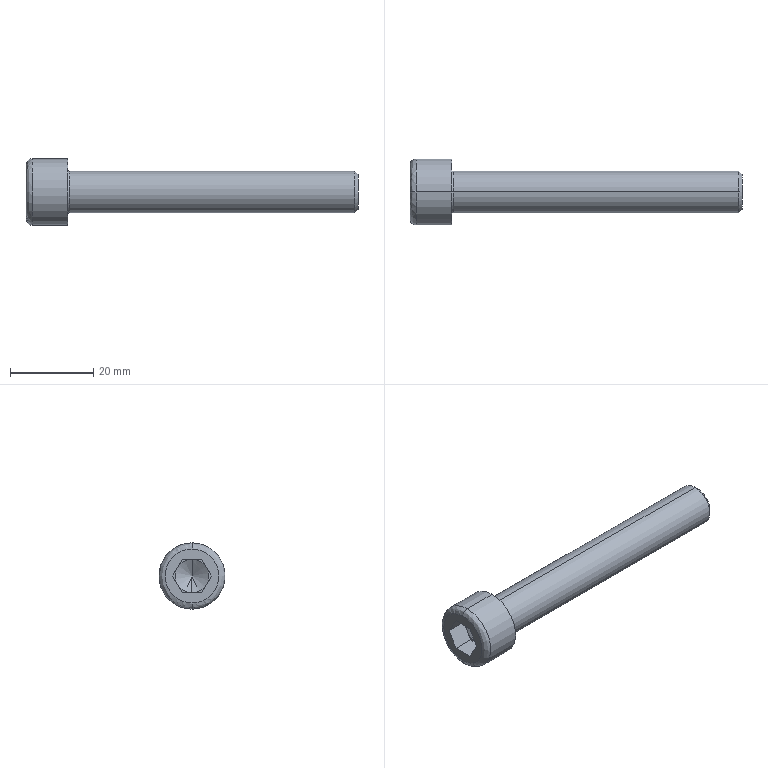Part | SolidWorks | features BaseBody 1 | 1 solid | 27 faces | box 80 x 16 x 16 mm | volume 7150 mm3 | plane 15 | spline 4 | cylinder 4 | cone 4 | commonest cylinder face diameters 10 x2 16 x2
STEP:
#1=CARTESIAN_POINT('',(10.,0.,5.4));
#2=VERTEX_POINT('',#1);
#3=CARTESIAN_POINT('',(10.,0.,-5.4));
#4=VERTEX_POINT('',#3);
#5=CARTESIAN_POINT('',(10.,0.,5.4));
#6=CARTESIAN_POINT('',(10.,0.1651,5.4));
#7=CARTESIAN_POINT('',(10.,0.4117,5.389));
#8=CARTESIAN_POINT('',(10.,0.6977,5.356));
#9=CARTESIAN_POINT('',(10.,0.8403,5.334));
#10=CARTESIAN_POINT('',(10.,0.9013,5.324));
#11=CARTESIAN_POINT('',(10.,0.942,5.317));
#12=CARTESIAN_POINT('',(10.,0.9611,5.314));
#13=CARTESIAN_POINT('',(10.,1.155,5.278));
#14=CARTESIAN_POINT('',(10.,1.409,5.218));
#15=CARTESIAN_POINT('',(10.,1.7,5.127));
#16=CARTESIAN_POINT('',(10.,1.824,5.083));
#17=CARTESIAN_POINT('',(10.,1.906,5.053));
#18=CARTESIAN_POINT('',(10.,1.945,5.038));
#19=CARTESIAN_POINT('',(10.,2.157,4.954));
#20=CARTESIAN_POINT('',(10.,2.405,4.841));
#21=CARTESIAN_POINT('',(10.,2.644,4.709));
#22=CARTESIAN_POINT('',(10.,2.801,4.618));
#23=CARTESIAN_POINT('',(10.,2.877,4.571));
#24=CARTESIAN_POINT('',(10.,3.267,4.316));
#25=CARTESIAN_POINT('',(10.,3.555,4.082));
#26=CARTESIAN_POINT('',(10.,3.95,3.687));
#27=CARTESIAN_POINT('',(10.,4.137,3.48));
#28=CARTESIAN_POINT('',(10.,4.306,3.26));
#29=CARTESIAN_POINT('',(10.,4.416,3.11));
#30=CARTESIAN_POINT('',(10.,4.47,3.031));
#31=CARTESIAN_POINT('',(10.,4.62,2.802));
#32=CARTESIAN_POINT('',(10.,4.757,2.567));
#33=CARTESIAN_POINT('',(10.,4.896,2.281));
#34=CARTESIAN_POINT('',(10.,4.951,2.156));
#35=CARTESIAN_POINT('',(10.,4.987,2.072));
#36=CARTESIAN_POINT('',(10.,5.005,2.028));
#37=CARTESIAN_POINT('',(10.,5.085,1.825));
#38=CARTESIAN_POINT('',(10.,5.17,1.577));
#39=CARTESIAN_POINT('',(10.,5.247,1.282));
#40=CARTESIAN_POINT('',(10.,5.28,1.133));
#41=CARTESIAN_POINT('',(10.,5.293,1.069));
#42=CARTESIAN_POINT('',(10.,5.302,1.026));
#43=CARTESIAN_POINT('',(10.,5.306,1.003));
#44=CARTESIAN_POINT('',(10.,5.37,0.6582));
#45=CARTESIAN_POINT('',(10.,5.4,0.3299));
#46=CARTESIAN_POINT('',(10.,5.4,-0.165));
#47=CARTESIAN_POINT('',(10.,5.389,-0.4115));
#48=CARTESIAN_POINT('',(10.,5.356,-0.6976));
#49=CARTESIAN_POINT('',(10.,5.335,-0.8402));
#50=CARTESIAN_POINT('',(10.,5.324,-0.9013));
#51=CARTESIAN_POINT('',(10.,5.317,-0.9419));
#52=CARTESIAN_POINT('',(10.,5.314,-0.9611));
#53=CARTESIAN_POINT('',(10.,5.278,-1.155));
#54=CARTESIAN_POINT('',(10.,5.218,-1.409));
#55=CARTESIAN_POINT('',(10.,5.127,-1.7));
#56=CARTESIAN_POINT('',(10.,5.083,-1.824));
#57=CARTESIAN_POINT('',(10.,5.053,-1.906));
#58=CARTESIAN_POINT('',(10.,5.038,-1.945));
#59=CARTESIAN_POINT('',(10.,4.954,-2.157));
#60=CARTESIAN_POINT('',(10.,4.841,-2.405));
#61=CARTESIAN_POINT('',(10.,4.709,-2.644));
#62=CARTESIAN_POINT('',(10.,4.618,-2.801));
#63=CARTESIAN_POINT('',(10.,4.571,-2.877));
#64=CARTESIAN_POINT('',(10.,4.316,-3.267));
#65=CARTESIAN_POINT('',(10.,4.082,-3.555));
#66=CARTESIAN_POINT('',(10.,3.687,-3.95));
#67=CARTESIAN_POINT('',(10.,3.48,-4.137));
#68=CARTESIAN_POINT('',(10.,3.26,-4.306));
#69=CARTESIAN_POINT('',(10.,3.11,-4.416));
#70=CARTESIAN_POINT('',(10.,3.031,-4.47));
#71=CARTESIAN_POINT('',(10.,2.802,-4.62));
#72=CARTESIAN_POINT('',(10.,2.567,-4.757));
#73=CARTESIAN_POINT('',(10.,2.281,-4.896));
#74=CARTESIAN_POINT('',(10.,2.156,-4.951));
#75=CARTESIAN_POINT('',(10.,2.072,-4.987));
#76=CARTESIAN_POINT('',(10.,2.028,-5.005));
#77=CARTESIAN_POINT('',(10.,1.825,-5.085));
#78=CARTESIAN_POINT('',(10.,1.577,-5.17));
#79=CARTESIAN_POINT('',(10.,1.282,-5.247));
#80=CARTESIAN_POINT('',(10.,1.133,-5.28));
#81=CARTESIAN_POINT('',(10.,1.069,-5.293));
#82=CARTESIAN_POINT('',(10.,1.026,-5.302));
#83=CARTESIAN_POINT('',(10.,1.003,-5.306));
#84=CARTESIAN_POINT('',(10.,0.658,-5.37));
#85=CARTESIAN_POINT('',(10.,0.3305,-5.4));
#86=CARTESIAN_POINT('',(10.,0.,-5.4));
#87=B_SPLINE_CURVE_WITH_KNOTS('',3,(#5,#6,#7,#8,#9,#10,#11,#12,#13,#14,#15,#16,#17,#18,#19,#20,#21,#22,#23,#24,#25,#26,#27,#28,#29,#30,#31,#32,#33,#34,#35,#36,#37,#38,#39,#40,#41,#42,#43,#44,#45,#46,#47,#48,#49,#50,#51,#52,#53,#54,#55,#56,#57,#58,#59,#60,#61,#62,#63,#64,#65,#66,#67,#68,#69,#70,#71,#72,#73,#74,#75,#76,#77,#78,#79,#80,#81,#82,#83,#84,#85,#86),.UNSPECIFIED.,.F.,.F.,(4,1,1,1,2,2,1,1,2,2,1,2,2,2,1,2,2,1,1,2,2,1,1,1,2,2,2,1,1,1,2,2,1,1,2,2,1,2,2,2,1,2,2,1,1,2,2,1,1,1,2,2,4),(0.,0.03125,0.04687,0.05469,0.05859,0.0625,0.09375,0.1094,0.1172,0.125,0.1562,0.1719,0.1875,0.25,0.2812,0.2969,0.3125,0.3437,0.3594,0.3672,0.375,0.4062,0.4219,0.4297,0.4336,0.4375,0.5,0.5312,0.5469,0.5547,0.5586,0.5625,0.5937,0.6094,0.6172,0.625,0.6562,0.6719,0.6875,0.75,0.7813,0.7969,0.8125,0.8438,0.8594,0.8672,0.875,0.9063,0.9219,0.9297,0.9336,0.9375,1.),.UNSPECIFIED.);
#88=EDGE_CURVE('',#2,#4,#87,.T.);
#89=ORIENTED_EDGE('',*,*,#88,.F.);
#90=CARTESIAN_POINT('',(10.4,0.,5.));
#91=VERTEX_POINT('',#90);
#92=CARTESIAN_POINT('',(10.4,0.,5.4));
#93=DIRECTION('',(0.,-1.,0.));
#94=DIRECTION('',(0.,0.,1.));
#95=AXIS2_PLACEMENT_3D('',#92,#93,#94);
#96=CIRCLE('',#95,0.4);
#97=EDGE_CURVE('',#2,#91,#96,.T.);
#98=ORIENTED_EDGE('',*,*,#97,.T.);
#99=CARTESIAN_POINT('',(10.4,0.,-5.));
#100=VERTEX_POINT('',#99);
#101=CARTESIAN_POINT('',(10.4,0.,0.));
#102=DIRECTION('',(1.,0.,0.));
#103=DIRECTION('',(0.,0.,1.));
#104=AXIS2_PLACEMENT_3D('',#101,#102,#103);
#105=CIRCLE('',#104,5.);
#106=EDGE_CURVE('',#100,#91,#105,.T.);
#107=ORIENTED_EDGE('',*,*,#106,.F.);
#108=CARTESIAN_POINT('',(10.4,0.,-5.4));
#109=DIRECTION('',(0.,1.,0.));
#110=DIRECTION('',(0.,0.,-1.));
#111=AXIS2_PLACEMENT_3D('',#108,#109,#110);
#112=CIRCLE('',#111,0.4);
#113=EDGE_CURVE('',#4,#100,#112,.T.);
#114=ORIENTED_EDGE('',*,*,#113,.F.);
#115=EDGE_LOOP('',(#89,#98,#107,#114));
#116=FACE_OUTER_BOUND('',#115,.T.);
#117=CARTESIAN_POINT('',(10.,0.,-5.4));
#118=CARTESIAN_POINT('',(10.,10.8,-5.4));
#119=CARTESIAN_POINT('',(10.,10.8,5.4));
#120=CARTESIAN_POINT('',(10.,0.,5.4));
#121=CARTESIAN_POINT('',(10.,0.,-5.166));
#122=CARTESIAN_POINT('',(10.,10.331,-5.166));
#123=CARTESIAN_POINT('',(10.,10.331,5.166));
#124=CARTESIAN_POINT('',(10.,0.,5.166));
#125=CARTESIAN_POINT('',(10.166,0.,-5.));
#126=CARTESIAN_POINT('',(10.166,10.,-5.));
#127=CARTESIAN_POINT('',(10.166,10.,5.));
#128=CARTESIAN_POINT('',(10.166,0.,5.));
#129=CARTESIAN_POINT('',(10.4,0.,-5.));
#130=CARTESIAN_POINT('',(10.4,10.,-5.));
#131=CARTESIAN_POINT('',(10.4,10.,5.));
#132=CARTESIAN_POINT('',(10.4,0.,5.));
#133=(BOUNDED_SURFACE()B_SPLINE_SURFACE(3,3,((#117,#118,#119,#120),(#121,#122,#123,#124),(#125,#126,#127,#128),(#129,#130,#131,#132)),.UNSPECIFIED.,.F.,.F.,.F.)B_SPLINE_SURFACE_WITH_KNOTS((4,4),(4,4),(0.,1.),(0.,1.),.UNSPECIFIED.)GEOMETRIC_REPRESENTATION_ITEM()RATIONAL_B_SPLINE_SURFACE(((1.,0.3333,0.3333,1.),(0.8047,0.2682,0.2682,0.8047),(0.8047,0.2682,0.2682,0.8047),(1.,0.3333,0.3333,1.)))REPRESENTATION_ITEM('')SURFACE());
#134=ADVANCED_FACE('',(#116),#133,.F.);
#135=CARTESIAN_POINT('',(0.,0.,6.5));
#136=VERTEX_POINT('',#135);
#137=CARTESIAN_POINT('',(0.,0.,-6.5));
#138=VERTEX_POINT('',#137);
#139=CARTESIAN_POINT('',(0.,0.,6.5));
#140=CARTESIAN_POINT('',(0.,-13.,6.5));
#141=CARTESIAN_POINT('',(0.,-13.,-6.5));
#142=CARTESIAN_POINT('',(0.,0.,-6.5));
#143=(BOUNDED_CURVE()B_SPLINE_CURVE(3,(#139,#140,#141,#142),.UNSPECIFIED.,.F.,.F.)B_SPLINE_CURVE_WITH_KNOTS((4,4),(0.,1.),.UNSPECIFIED.)CURVE()GEOMETRIC_REPRESENTATION_ITEM()RATIONAL_B_SPLINE_CURVE((1.,0.3333,0.3333,1.))REPRESENTATION_ITEM(''));
#144=EDGE_CURVE('',#136,#138,#143,.T.);
#145=ORIENTED_EDGE('',*,*,#144,.T.);
#146=CARTESIAN_POINT('',(1.5,0.,-8.));
#147=VERTEX_POINT('',#146);
#148=CARTESIAN_POINT('',(1.5,0.,-6.5));
#149=DIRECTION('',(0.,-1.,0.));
#150=DIRECTION('',(0.,0.,-1.));
#151=AXIS2_PLACEMENT_3D('',#148,#149,#150);
#152=CIRCLE('',#151,1.5);
#153=EDGE_CURVE('',#138,#147,#152,.T.);
#154=ORIENTED_EDGE('',*,*,#153,.T.);
#155=CARTESIAN_POINT('',(1.5,0.,8.));
#156=VERTEX_POINT('',#155);
#157=CARTESIAN_POINT('',(1.5,0.,0.));
#158=DIRECTION('',(1.,0.,0.));
#159=DIRECTION('',(0.,0.,1.));
#160=AXIS2_PLACEMENT_3D('',#157,#158,#159);
#161=CIRCLE('',#160,8.);
#162=EDGE_CURVE('',#156,#147,#161,.T.);
#163=ORIENTED_EDGE('',*,*,#162,.F.);
#164=CARTESIAN_POINT('',(1.5,0.,6.5));
#165=DIRECTION('',(0.,1.,0.));
#166=DIRECTION('',(0.,0.,1.));
#167=AXIS2_PLACEMENT_3D('',#164,#165,#166);
#168=CIRCLE('',#167,1.5);
#169=EDGE_CURVE('',#136,#156,#168,.T.);
#170=ORIENTED_EDGE('',*,*,#169,.F.);
#171=EDGE_LOOP('',(#145,#154,#163,#170));
#172=FACE_OUTER_BOUND('',#171,.T.);
#173=CARTESIAN_POINT('',(0.,0.,-6.5));
#174=CARTESIAN_POINT('',(0.,-13.,-6.5));
#175=CARTESIAN_POINT('',(0.,-13.,6.5));
#176=CARTESIAN_POINT('',(0.,0.,6.5));
#177=CARTESIAN_POINT('',(0.,0.,-7.379));
#178=CARTESIAN_POINT('',(0.,-14.757,-7.379));
#179=CARTESIAN_POINT('',(0.,-14.757,7.379));
#180=CARTESIAN_POINT('',(0.,0.,7.379));
#181=CARTESIAN_POINT('',(0.6213,0.,-8.));
#182=CARTESIAN_POINT('',(0.6213,-16.,-8.));
#183=CARTESIAN_POINT('',(0.6213,-16.,8.));
#184=CARTESIAN_POINT('',(0.6213,0.,8.));
#185=CARTESIAN_POINT('',(1.5,0.,-8.));
#186=CARTESIAN_POINT('',(1.5,-16.,-8.));
#187=CARTESIAN_POINT('',(1.5,-16.,8.));
#188=CARTESIAN_POINT('',(1.5,0.,8.));
#189=(BOUNDED_SURFACE()B_SPLINE_SURFACE(3,3,((#173,#174,#175,#176),(#177,#178,#179,#180),(#181,#182,#183,#184),(#185,#186,#187,#188)),.UNSPECIFIED.,.F.,.F.,.F.)B_SPLINE_SURFACE_WITH_KNOTS((4,4),(4,4),(0.,1.),(0.,1.),.UNSPECIFIED.)GEOMETRIC_REPRESENTATION_ITEM()RATIONAL_B_SPLINE_SURFACE(((1.,0.3333,0.3333,1.),(0.8047,0.2682,0.2682,0.8047),(0.8047,0.2682,0.2682,0.8047),(1.,0.3333,0.3333,1.)))REPRESENTATION_ITEM('')SURFACE());
#190=ADVANCED_FACE('',(#172),#189,.T.);
#191=CARTESIAN_POINT('',(79.172,0.,5.));
#192=VERTEX_POINT('',#191);
#193=CARTESIAN_POINT('',(79.172,0.,-5.));
#194=VERTEX_POINT('',#193);
#195=CARTESIAN_POINT('',(79.172,0.,0.));
#196=DIRECTION('',(-1.,0.,0.));
#197=DIRECTION('',(0.,0.,1.));
#198=AXIS2_PLACEMENT_3D('',#195,#196,#197);
#199=CIRCLE('',#198,5.);
#200=EDGE_CURVE('',#192,#194,#199,.T.);
#201=ORIENTED_EDGE('',*,*,#200,.T.);
#202=CARTESIAN_POINT('',(-31.75,0.,-5.));
#203=DIRECTION('',(-1.,0.,0.));
#204=VECTOR('',#203,1000.);
#205=LINE('',#202,#204);
#206=EDGE_CURVE('',#194,#100,#205,.T.);
#207=ORIENTED_EDGE('',*,*,#206,.T.);
#208=ORIENTED_EDGE('',*,*,#106,.T.);
#209=CARTESIAN_POINT('',(-31.75,0.,5.));
#210=DIRECTION('',(-1.,0.,0.));
#211=VECTOR('',#210,1000.);
#212=LINE('',#209,#211);
#213=EDGE_CURVE('',#192,#91,#212,.T.);
#214=ORIENTED_EDGE('',*,*,#213,.F.);
#215=EDGE_LOOP('',(#201,#207,#208,#214));
#216=FACE_OUTER_BOUND('',#215,.T.);
#217=CARTESIAN_POINT('',(-31.75,0.,0.));
#218=DIRECTION('',(-1.,0.,0.));
#219=DIRECTION('',(0.,0.,1.));
#220=AXIS2_PLACEMENT_3D('',#217,#218,#219);
#221=CYLINDRICAL_SURFACE('',#220,5.);
#222=ADVANCED_FACE('',(#216),#221,.T.);
#223=CARTESIAN_POINT('',(80.,0.,4.172));
#224=VERTEX_POINT('',#223);
#225=CARTESIAN_POINT('',(80.,0.,-4.172));
#226=VERTEX_POINT('',#225);
#227=CARTESIAN_POINT('',(80.,0.,0.));
#228=DIRECTION('',(-1.,0.,0.));
#229=DIRECTION('',(0.,0.,1.));
#230=AXIS2_PLACEMENT_3D('',#227,#228,#229);
#231=CIRCLE('',#230,4.172);
#232=EDGE_CURVE('',#224,#226,#231,.T.);
#233=ORIENTED_EDGE('',*,*,#232,.T.);
#234=CARTESIAN_POINT('',(79.172,0.,-5.));
#235=DIRECTION('',(-0.7071,0.,-0.7071));
#236=VECTOR('',#235,1000.);
#237=LINE('',#234,#236);
#238=EDGE_CURVE('',#226,#194,#237,.T.);
#239=ORIENTED_EDGE('',*,*,#238,.T.);
#240=ORIENTED_EDGE('',*,*,#200,.F.);
#241=CARTESIAN_POINT('',(79.172,0.,5.));
#242=DIRECTION('',(-0.7071,0.,0.7071));
#243=VECTOR('',#242,1000.);
#244=LINE('',#241,#243);
#245=EDGE_CURVE('',#224,#192,#244,.T.);
#246=ORIENTED_EDGE('',*,*,#245,.F.);
#247=EDGE_LOOP('',(#233,#239,#240,#246));
#248=FACE_OUTER_BOUND('',#247,.T.);
#249=CARTESIAN_POINT('',(79.172,0.,0.));
#250=DIRECTION('',(-1.,0.,0.));
#251=DIRECTION('',(0.,0.,1.));
#252=AXIS2_PLACEMENT_3D('',#249,#250,#251);
#253=CONICAL_SURFACE('',#252,5.,0.7854);
#254=ADVANCED_FACE('',(#248),#253,.T.);
#255=CARTESIAN_POINT('',(10.,0.,-8.));
#256=VERTEX_POINT('',#255);
#257=CARTESIAN_POINT('',(10.,0.,8.));
#258=VERTEX_POINT('',#257);
#259=CARTESIAN_POINT('',(10.,0.,0.));
#260=DIRECTION('',(1.,0.,0.));
#261=DIRECTION('',(0.,0.,1.));
#262=AXIS2_PLACEMENT_3D('',#259,#260,#261);
#263=CIRCLE('',#262,8.);
#264=EDGE_CURVE('',#256,#258,#263,.T.);
#265=ORIENTED_EDGE('',*,*,#264,.F.);
#266=CARTESIAN_POINT('',(-31.75,0.,-8.));
#267=DIRECTION('',(-1.,0.,0.));
#268=VECTOR('',#267,1000.);
#269=LINE('',#266,#268);
#270=EDGE_CURVE('',#256,#147,#269,.T.);
#271=ORIENTED_EDGE('',*,*,#270,.T.);
#272=CARTESIAN_POINT('',(1.5,0.,0.));
#273=DIRECTION('',(1.,0.,0.));
#274=DIRECTION('',(0.,0.,1.));
#275=AXIS2_PLACEMENT_3D('',#272,#273,#274);
#276=CIRCLE('',#275,8.);
#277=EDGE_CURVE('',#147,#156,#276,.T.);
#278=ORIENTED_EDGE('',*,*,#277,.T.);
#279=CARTESIAN_POINT('',(-31.75,0.,8.));
#280=DIRECTION('',(-1.,0.,0.));
#281=VECTOR('',#280,1000.);
#282=LINE('',#279,#281);
#283=EDGE_CURVE('',#258,#156,#282,.T.);
#284=ORIENTED_EDGE('',*,*,#283,.F.);
#285=EDGE_LOOP('',(#265,#271,#278,#284));
#286=FACE_OUTER_BOUND('',#285,.T.);
#287=CARTESIAN_POINT('',(-31.75,0.,0.));
#288=DIRECTION('',(-1.,0.,0.));
#289=DIRECTION('',(0.,0.,1.));
#290=AXIS2_PLACEMENT_3D('',#287,#288,#289);
#291=CYLINDRICAL_SURFACE('',#290,8.);
#292=ADVANCED_FACE('',(#286),#291,.T.);
#293=CARTESIAN_POINT('',(7.343,0.,0.));
#294=VERTEX_POINT('',#293);
#295=CARTESIAN_POINT('',(5.,0.,4.057));
#296=VERTEX_POINT('',#295);
#297=CARTESIAN_POINT('',(5.,0.,4.057));
#298=DIRECTION('',(-0.5,0.,0.866));
#299=VECTOR('',#298,1000.);
#300=LINE('',#297,#299);
#301=EDGE_CURVE('',#294,#296,#300,.T.);
#302=ORIENTED_EDGE('',*,*,#301,.F.);
#303=CARTESIAN_POINT('',(5.,0.,-4.057));
#304=VERTEX_POINT('',#303);
#305=CARTESIAN_POINT('',(5.,0.,-4.057));
#306=DIRECTION('',(-0.5,0.,-0.866));
#307=VECTOR('',#306,1000.);
#308=LINE('',#305,#307);
#309=EDGE_CURVE('',#294,#304,#308,.T.);
#310=ORIENTED_EDGE('',*,*,#309,.T.);
#311=CARTESIAN_POINT('',(5.,-3.514,-2.029));
#312=VERTEX_POINT('',#311);
#313=CARTESIAN_POINT('',(5.,0.,0.));
#314=DIRECTION('',(-1.,0.,0.));
#315=DIRECTION('',(0.,0.,1.));
#316=AXIS2_PLACEMENT_3D('',#313,#314,#315);
#317=CIRCLE('',#316,4.057);
#318=EDGE_CURVE('',#304,#312,#317,.T.);
#319=ORIENTED_EDGE('',*,*,#318,.T.);
#320=CARTESIAN_POINT('',(5.,-3.514,2.029));
#321=VERTEX_POINT('',#320);
#322=CARTESIAN_POINT('',(5.,0.,0.));
#323=DIRECTION('',(-1.,0.,0.));
#324=DIRECTION('',(0.,0.,1.));
#325=AXIS2_PLACEMENT_3D('',#322,#323,#324);
#326=CIRCLE('',#325,4.057);
#327=EDGE_CURVE('',#312,#321,#326,.T.);
#328=ORIENTED_EDGE('',*,*,#327,.T.);
#329=CARTESIAN_POINT('',(5.,0.,0.));
#330=DIRECTION('',(-1.,0.,0.));
#331=DIRECTION('',(0.,0.,1.));
#332=AXIS2_PLACEMENT_3D('',#329,#330,#331);
#333=CIRCLE('',#332,4.057);
#334=EDGE_CURVE('',#321,#296,#333,.T.);
#335=ORIENTED_EDGE('',*,*,#334,.T.);
#336=EDGE_LOOP('',(#302,#310,#319,#328,#335));
#337=FACE_OUTER_BOUND('',#336,.T.);
#338=CARTESIAN_POINT('',(5.,0.,0.));
#339=DIRECTION('',(-1.,0.,0.));
#340=DIRECTION('',(0.,0.,1.));
#341=AXIS2_PLACEMENT_3D('',#338,#339,#340);
#342=CONICAL_SURFACE('',#341,4.057,1.047);
#343=ADVANCED_FACE('',(#337),#342,.F.);
#344=ORIENTED_EDGE('',*,*,#206,.F.);
#345=CARTESIAN_POINT('',(79.172,0.,0.));
#346=DIRECTION('',(-1.,0.,0.));
#347=DIRECTION('',(0.,0.,1.));
#348=AXIS2_PLACEMENT_3D('',#345,#346,#347);
#349=CIRCLE('',#348,5.);
#350=EDGE_CURVE('',#194,#192,#349,.T.);
#351=ORIENTED_EDGE('',*,*,#350,.T.);
#352=ORIENTED_EDGE('',*,*,#213,.T.);
#353=CARTESIAN_POINT('',(10.4,0.,0.));
#354=DIRECTION('',(1.,0.,0.));
#355=DIRECTION('',(0.,0.,1.));
#356=AXIS2_PLACEMENT_3D('',#353,#354,#355);
#357=CIRCLE('',#356,5.);
#358=EDGE_CURVE('',#91,#100,#357,.T.);
#359=ORIENTED_EDGE('',*,*,#358,.T.);
#360=EDGE_LOOP('',(#344,#351,#352,#359));
#361=FACE_OUTER_BOUND('',#360,.T.);
#362=CARTESIAN_POINT('',(-31.75,0.,0.));
#363=DIRECTION('',(-1.,0.,0.));
#364=DIRECTION('',(0.,0.,1.));
#365=AXIS2_PLACEMENT_3D('',#362,#363,#364);
#366=CYLINDRICAL_SURFACE('',#365,5.);
#367=ADVANCED_FACE('',(#361),#366,.T.);
#368=ORIENTED_EDGE('',*,*,#97,.F.);
#369=CARTESIAN_POINT('',(10.,0.,-5.4));
#370=CARTESIAN_POINT('',(10.,-0.1651,-5.4));
#371=CARTESIAN_POINT('',(10.,-0.4117,-5.389));
#372=CARTESIAN_POINT('',(10.,-0.6977,-5.356));
#373=CARTESIAN_POINT('',(10.,-0.8403,-5.334));
#374=CARTESIAN_POINT('',(10.,-0.9013,-5.324));
#375=CARTESIAN_POINT('',(10.,-0.942,-5.317));
#376=CARTESIAN_POINT('',(10.,-0.9611,-5.314));
#377=CARTESIAN_POINT('',(10.,-1.155,-5.278));
#378=CARTESIAN_POINT('',(10.,-1.409,-5.218));
#379=CARTESIAN_POINT('',(10.,-1.7,-5.127));
#380=CARTESIAN_POINT('',(10.,-1.824,-5.083));
#381=CARTESIAN_POINT('',(10.,-1.906,-5.053));
#382=CARTESIAN_POINT('',(10.,-1.945,-5.038));
#383=CARTESIAN_POINT('',(10.,-2.157,-4.954));
#384=CARTESIAN_POINT('',(10.,-2.405,-4.841));
#385=CARTESIAN_POINT('',(10.,-2.644,-4.709));
#386=CARTESIAN_POINT('',(10.,-2.801,-4.618));
#387=CARTESIAN_POINT('',(10.,-2.877,-4.571));
#388=CARTESIAN_POINT('',(10.,-3.267,-4.316));
#389=CARTESIAN_POINT('',(10.,-3.555,-4.082));
#390=CARTESIAN_POINT('',(10.,-3.95,-3.687));
#391=CARTESIAN_POINT('',(10.,-4.137,-3.48));
#392=CARTESIAN_POINT('',(10.,-4.306,-3.26));
#393=CARTESIAN_POINT('',(10.,-4.416,-3.11));
#394=CARTESIAN_POINT('',(10.,-4.47,-3.031));
#395=CARTESIAN_POINT('',(10.,-4.62,-2.802));
#396=CARTESIAN_POINT('',(10.,-4.757,-2.567));
#397=CARTESIAN_POINT('',(10.,-4.896,-2.281));
#398=CARTESIAN_POINT('',(10.,-4.951,-2.156));
#399=CARTESIAN_POINT('',(10.,-4.987,-2.072));
#400=CARTESIAN_POINT('',(10.,-5.005,-2.028));
#401=CARTESIAN_POINT('',(10.,-5.085,-1.825));
#402=CARTESIAN_POINT('',(10.,-5.17,-1.577));
#403=CARTESIAN_POINT('',(10.,-5.247,-1.282));
#404=CARTESIAN_POINT('',(10.,-5.28,-1.133));
#405=CARTESIAN_POINT('',(10.,-5.293,-1.069));
#406=CARTESIAN_POINT('',(10.,-5.302,-1.026));
#407=CARTESIAN_POINT('',(10.,-5.306,-1.003));
#408=CARTESIAN_POINT('',(10.,-5.37,-0.6582));
#409=CARTESIAN_POINT('',(10.,-5.4,-0.3299));
#410=CARTESIAN_POINT('',(10.,-5.4,0.165));
#411=CARTESIAN_POINT('',(10.,-5.389,0.4115));
#412=CARTESIAN_POINT('',(10.,-5.356,0.6976));
#413=CARTESIAN_POINT('',(10.,-5.335,0.8402));
#414=CARTESIAN_POINT('',(10.,-5.324,0.9013));
#415=CARTESIAN_POINT('',(10.,-5.317,0.9419));
#416=CARTESIAN_POINT('',(10.,-5.314,0.9611));
#417=CARTESIAN_POINT('',(10.,-5.278,1.155));
#418=CARTESIAN_POINT('',(10.,-5.218,1.409));
#419=CARTESIAN_POINT('',(10.,-5.127,1.7));
#420=CARTESIAN_POINT('',(10.,-5.083,1.824));
#421=CARTESIAN_POINT('',(10.,-5.053,1.906));
#422=CARTESIAN_POINT('',(10.,-5.038,1.945));
#423=CARTESIAN_POINT('',(10.,-4.954,2.157));
#424=CARTESIAN_POINT('',(10.,-4.841,2.405));
#425=CARTESIAN_POINT('',(10.,-4.709,2.644));
#426=CARTESIAN_POINT('',(10.,-4.618,2.801));
#427=CARTESIAN_POINT('',(10.,-4.571,2.877));
#428=CARTESIAN_POINT('',(10.,-4.316,3.267));
#429=CARTESIAN_POINT('',(10.,-4.082,3.555));
#430=CARTESIAN_POINT('',(10.,-3.687,3.95));
#431=CARTESIAN_POINT('',(10.,-3.48,4.137));
#432=CARTESIAN_POINT('',(10.,-3.26,4.306));
#433=CARTESIAN_POINT('',(10.,-3.11,4.416));
#434=CARTESIAN_POINT('',(10.,-3.031,4.47));
#435=CARTESIAN_POINT('',(10.,-2.802,4.62));
#436=CARTESIAN_POINT('',(10.,-2.567,4.757));
#437=CARTESIAN_POINT('',(10.,-2.281,4.896));
#438=CARTESIAN_POINT('',(10.,-2.156,4.951));
#439=CARTESIAN_POINT('',(10.,-2.072,4.987));
#440=CARTESIAN_POINT('',(10.,-2.028,5.005));
#441=CARTESIAN_POINT('',(10.,-1.825,5.085));
#442=CARTESIAN_POINT('',(10.,-1.577,5.17));
#443=CARTESIAN_POINT('',(10.,-1.282,5.247));
#444=CARTESIAN_POINT('',(10.,-1.133,5.28));
#445=CARTESIAN_POINT('',(10.,-1.069,5.293));
#446=CARTESIAN_POINT('',(10.,-1.026,5.302));
#447=CARTESIAN_POINT('',(10.,-1.003,5.306));
#448=CARTESIAN_POINT('',(10.,-0.658,5.37));
#449=CARTESIAN_POINT('',(10.,-0.3305,5.4));
#450=CARTESIAN_POINT('',(10.,0.,5.4));
#451=B_SPLINE_CURVE_WITH_KNOTS('',3,(#369,#370,#371,#372,#373,#374,#375,#376,#377,#378,#379,#380,#381,#382,#383,#384,#385,#386,#387,#388,#389,#390,#391,#392,#393,#394,#395,#396,#397,#398,#399,#400,#401,#402,#403,#404,#405,#406,#407,#408,#409,#410,#411,#412,#413,#414,#415,#416,#417,#418,#419,#420,#421,#422,#423,#424,#425,#426,#427,#428,#429,#430,#431,#432,#433,#434,#435,#436,#437,#438,#439,#440,#441,#442,#443,#444,#445,#446,#447,#448,#449,#450),.UNSPECIFIED.,.F.,.F.,(4,1,1,1,2,2,1,1,2,2,1,2,2,2,1,2,2,1,1,2,2,1,1,1,2,2,2,1,1,1,2,2,1,1,2,2,1,2,2,2,1,2,2,1,1,2,2,1,1,1,2,2,4),(0.,0.03125,0.04687,0.05469,0.05859,0.0625,0.09375,0.1094,0.1172,0.125,0.1562,0.1719,0.1875,0.25,0.2813,0.2969,0.3125,0.3438,0.3594,0.3672,0.375,0.4063,0.4219,0.4297,0.4336,0.4375,0.5,0.5313,0.5469,0.5547,0.5586,0.5625,0.5938,0.6094,0.6172,0.625,0.6563,0.6719,0.6875,0.75,0.7813,0.7969,0.8125,0.8438,0.8594,0.8672,0.875,0.9063,0.9219,0.9297,0.9336,0.9375,1.),.UNSPECIFIED.);
#452=EDGE_CURVE('',#4,#2,#451,.T.);
#453=ORIENTED_EDGE('',*,*,#452,.F.);
#454=ORIENTED_EDGE('',*,*,#113,.T.);
#455=ORIENTED_EDGE('',*,*,#358,.F.);
#456=EDGE_LOOP('',(#368,#453,#454,#455));
#457=FACE_OUTER_BOUND('',#456,.T.);
#458=CARTESIAN_POINT('',(10.,0.,5.4));
#459=CARTESIAN_POINT('',(10.,-10.8,5.4));
#460=CARTESIAN_POINT('',(10.,-10.8,-5.4));
#461=CARTESIAN_POINT('',(10.,0.,-5.4));
#462=CARTESIAN_POINT('',(10.,0.,5.166));
#463=CARTESIAN_POINT('',(10.,-10.331,5.166));
#464=CARTESIAN_POINT('',(10.,-10.331,-5.166));
#465=CARTESIAN_POINT('',(10.,0.,-5.166));
#466=CARTESIAN_POINT('',(10.166,0.,5.));
#467=CARTESIAN_POINT('',(10.166,-10.,5.));
#468=CARTESIAN_POINT('',(10.166,-10.,-5.));
#469=CARTESIAN_POINT('',(10.166,0.,-5.));
#470=CARTESIAN_POINT('',(10.4,0.,5.));
#471=CARTESIAN_POINT('',(10.4,-10.,5.));
#472=CARTESIAN_POINT('',(10.4,-10.,-5.));
#473=CARTESIAN_POINT('',(10.4,0.,-5.));
#474=(BOUNDED_SURFACE()B_SPLINE_SURFACE(3,3,((#458,#459,#460,#461),(#462,#463,#464,#465),(#466,#467,#468,#469),(#470,#471,#472,#473)),.UNSPECIFIED.,.F.,.F.,.T.)B_SPLINE_SURFACE_WITH_KNOTS((4,4),(4,4),(0.,1.),(0.,1.),.UNSPECIFIED.)GEOMETRIC_REPRESENTATION_ITEM()RATIONAL_B_SPLINE_SURFACE(((1.,0.3333,0.3333,1.),(0.8047,0.2682,0.2682,0.8047),(0.8047,0.2682,0.2682,0.8047),(1.,0.3333,0.3333,1.)))REPRESENTATION_ITEM('')SURFACE());
#475=ADVANCED_FACE('',(#457),#474,.F.);
#476=ORIENTED_EDGE('',*,*,#238,.F.);
#477=CARTESIAN_POINT('',(80.,0.,0.));
#478=DIRECTION('',(-1.,0.,0.));
#479=DIRECTION('',(0.,0.,1.));
#480=AXIS2_PLACEMENT_3D('',#477,#478,#479);
#481=CIRCLE('',#480,4.172);
#482=EDGE_CURVE('',#226,#224,#481,.T.);
#483=ORIENTED_EDGE('',*,*,#482,.T.);
#484=ORIENTED_EDGE('',*,*,#245,.T.);
#485=ORIENTED_EDGE('',*,*,#350,.F.);
#486=EDGE_LOOP('',(#476,#483,#484,#485));
#487=FACE_OUTER_BOUND('',#486,.T.);
#488=CARTESIAN_POINT('',(79.172,0.,0.));
#489=DIRECTION('',(-1.,0.,0.));
#490=DIRECTION('',(0.,0.,1.));
#491=AXIS2_PLACEMENT_3D('',#488,#489,#490);
#492=CONICAL_SURFACE('',#491,5.,0.7854);
#493=ADVANCED_FACE('',(#487),#492,.T.);
#494=CARTESIAN_POINT('',(10.,0.,0.));
#495=DIRECTION('',(1.,0.,0.));
#496=DIRECTION('',(0.,0.,1.));
#497=AXIS2_PLACEMENT_3D('',#494,#495,#496);
#498=CIRCLE('',#497,8.);
#499=EDGE_CURVE('',#258,#256,#498,.T.);
#500=ORIENTED_EDGE('',*,*,#499,.T.);
#501=ORIENTED_EDGE('',*,*,#264,.T.);
#502=EDGE_LOOP('',(#500,#501));
#503=FACE_OUTER_BOUND('',#502,.T.);
#504=ORIENTED_EDGE('',*,*,#452,.T.);
#505=ORIENTED_EDGE('',*,*,#88,.T.);
#506=EDGE_LOOP('',(#504,#505));
#507=FACE_BOUND('',#506,.T.);
#508=CARTESIAN_POINT('',(10.,8.,0.));
#509=DIRECTION('',(1.,0.,0.));
#510=DIRECTION('',(0.,0.,-1.));
#511=AXIS2_PLACEMENT_3D('',#508,#509,#510);
#512=PLANE('',#511);
#513=ADVANCED_FACE('',(#503,#507),#512,.T.);
#514=ORIENTED_EDGE('',*,*,#232,.F.);
#515=ORIENTED_EDGE('',*,*,#482,.F.);
#516=EDGE_LOOP('',(#514,#515));
#517=FACE_OUTER_BOUND('',#516,.T.);
#518=CARTESIAN_POINT('',(80.,4.172,0.));
#519=DIRECTION('',(1.,0.,0.));
#520=DIRECTION('',(0.,0.,-1.));
#521=AXIS2_PLACEMENT_3D('',#518,#519,#520);
#522=PLANE('',#521);
#523=ADVANCED_FACE('',(#517),#522,.T.);
#524=ORIENTED_EDGE('',*,*,#270,.F.);
#525=ORIENTED_EDGE('',*,*,#499,.F.);
#526=ORIENTED_EDGE('',*,*,#283,.T.);
#527=ORIENTED_EDGE('',*,*,#162,.T.);
#528=EDGE_LOOP('',(#524,#525,#526,#527));
#529=FACE_OUTER_BOUND('',#528,.T.);
#530=CARTESIAN_POINT('',(-31.75,0.,0.));
#531=DIRECTION('',(-1.,0.,0.));
#532=DIRECTION('',(0.,0.,1.));
#533=AXIS2_PLACEMENT_3D('',#530,#531,#532);
#534=CYLINDRICAL_SURFACE('',#533,8.);
#535=ADVANCED_FACE('',(#529),#534,.T.);
#536=ORIENTED_EDGE('',*,*,#153,.F.);
#537=CARTESIAN_POINT('',(0.,0.,-6.5));
#538=CARTESIAN_POINT('',(0.,13.,-6.5));
#539=CARTESIAN_POINT('',(0.,13.,6.5));
#540=CARTESIAN_POINT('',(0.,0.,6.5));
#541=(BOUNDED_CURVE()B_SPLINE_CURVE(3,(#537,#538,#539,#540),.UNSPECIFIED.,.F.,.F.)B_SPLINE_CURVE_WITH_KNOTS((4,4),(0.,1.),.UNSPECIFIED.)CURVE()GEOMETRIC_REPRESENTATION_ITEM()RATIONAL_B_SPLINE_CURVE((1.,0.3333,0.3333,1.))REPRESENTATION_ITEM(''));
#542=EDGE_CURVE('',#138,#136,#541,.T.);
#543=ORIENTED_EDGE('',*,*,#542,.T.);
#544=ORIENTED_EDGE('',*,*,#169,.T.);
#545=ORIENTED_EDGE('',*,*,#277,.F.);
#546=EDGE_LOOP('',(#536,#543,#544,#545));
#547=FACE_OUTER_BOUND('',#546,.T.);
#548=CARTESIAN_POINT('',(0.,0.,6.5));
#549=CARTESIAN_POINT('',(0.,13.,6.5));
#550=CARTESIAN_POINT('',(0.,13.,-6.5));
#551=CARTESIAN_POINT('',(0.,0.,-6.5));
#552=CARTESIAN_POINT('',(0.,0.,7.379));
#553=CARTESIAN_POINT('',(0.,14.757,7.379));
#554=CARTESIAN_POINT('',(0.,14.757,-7.379));
#555=CARTESIAN_POINT('',(0.,0.,-7.379));
#556=CARTESIAN_POINT('',(0.6213,0.,8.));
#557=CARTESIAN_POINT('',(0.6213,16.,8.));
#558=CARTESIAN_POINT('',(0.6213,16.,-8.));
#559=CARTESIAN_POINT('',(0.6213,0.,-8.));
#560=CARTESIAN_POINT('',(1.5,0.,8.));
#561=CARTESIAN_POINT('',(1.5,16.,8.));
#562=CARTESIAN_POINT('',(1.5,16.,-8.));
#563=CARTESIAN_POINT('',(1.5,0.,-8.));
#564=(BOUNDED_SURFACE()B_SPLINE_SURFACE(3,3,((#548,#549,#550,#551),(#552,#553,#554,#555),(#556,#557,#558,#559),(#560,#561,#562,#563)),.UNSPECIFIED.,.F.,.F.,.F.)B_SPLINE_SURFACE_WITH_KNOTS((4,4),(4,4),(0.,1.),(0.,1.),.UNSPECIFIED.)GEOMETRIC_REPRESENTATION_ITEM()RATIONAL_B_SPLINE_SURFACE(((1.,0.3333,0.3333,1.),(0.8047,0.2682,0.2682,0.8047),(0.8047,0.2682,0.2682,0.8047),(1.,0.3333,0.3333,1.)))REPRESENTATION_ITEM('')SURFACE());
#565=ADVANCED_FACE('',(#547),#564,.T.);
#566=ORIENTED_EDGE('',*,*,#542,.F.);
#567=ORIENTED_EDGE('',*,*,#144,.F.);
#568=EDGE_LOOP('',(#566,#567));
#569=FACE_OUTER_BOUND('',#568,.T.);
#570=CARTESIAN_POINT('',(0.,-2.343,-4.058));
#571=VERTEX_POINT('',#570);
#572=CARTESIAN_POINT('',(0.,2.343,-4.058));
#573=VERTEX_POINT('',#572);
#574=CARTESIAN_POINT('',(0.,0.,-4.058));
#575=DIRECTION('',(0.,1.,0.));
#576=VECTOR('',#575,1000.);
#577=LINE('',#574,#576);
#578=EDGE_CURVE('',#571,#573,#577,.T.);
#579=ORIENTED_EDGE('',*,*,#578,.T.);
#580=CARTESIAN_POINT('',(0.,4.685,0.));
#581=VERTEX_POINT('',#580);
#582=CARTESIAN_POINT('',(0.,2.343,-4.058));
#583=DIRECTION('',(0.,0.5,0.866));
#584=VECTOR('',#583,1000.);
#585=LINE('',#582,#584);
#586=EDGE_CURVE('',#573,#581,#585,.T.);
#587=ORIENTED_EDGE('',*,*,#586,.T.);
#588=CARTESIAN_POINT('',(0.,2.343,4.057));
#589=VERTEX_POINT('',#588);
#590=CARTESIAN_POINT('',(0.,4.685,0.));
#591=DIRECTION('',(0.,-0.5,0.866));
#592=VECTOR('',#591,1000.);
#593=LINE('',#590,#592);
#594=EDGE_CURVE('',#581,#589,#593,.T.);
#595=ORIENTED_EDGE('',*,*,#594,.T.);
#596=CARTESIAN_POINT('',(0.,-2.343,4.057));
#597=VERTEX_POINT('',#596);
#598=CARTESIAN_POINT('',(0.,0.,4.057));
#599=DIRECTION('',(0.,-1.,0.));
#600=VECTOR('',#599,1000.);
#601=LINE('',#598,#600);
#602=EDGE_CURVE('',#589,#597,#601,.T.);
#603=ORIENTED_EDGE('',*,*,#602,.T.);
#604=CARTESIAN_POINT('',(0.,-4.685,0.));
#605=VERTEX_POINT('',#604);
#606=CARTESIAN_POINT('',(0.,-2.343,4.058));
#607=DIRECTION('',(0.,-0.5,-0.866));
#608=VECTOR('',#607,1000.);
#609=LINE('',#606,#608);
#610=EDGE_CURVE('',#597,#605,#609,.T.);
#611=ORIENTED_EDGE('',*,*,#610,.T.);
#612=CARTESIAN_POINT('',(0.,-4.685,0.));
#613=DIRECTION('',(0.,0.5,-0.866));
#614=VECTOR('',#613,1000.);
#615=LINE('',#612,#614);
#616=EDGE_CURVE('',#605,#571,#615,.T.);
#617=ORIENTED_EDGE('',*,*,#616,.T.);
#618=EDGE_LOOP('',(#579,#587,#595,#603,#611,#617));
#619=FACE_BOUND('',#618,.T.);
#620=CARTESIAN_POINT('',(0.,0.,0.));
#621=DIRECTION('',(-1.,0.,0.));
#622=DIRECTION('',(0.,0.,1.));
#623=AXIS2_PLACEMENT_3D('',#620,#621,#622);
#624=PLANE('',#623);
#625=ADVANCED_FACE('',(#569,#619),#624,.T.);
#626=CARTESIAN_POINT('',(5.,2.343,-4.058));
#627=VERTEX_POINT('',#626);
#628=CARTESIAN_POINT('',(5.,2.343,-4.058));
#629=DIRECTION('',(-1.,0.,0.));
#630=VECTOR('',#629,1000.);
#631=LINE('',#628,#630);
#632=EDGE_CURVE('',#627,#573,#631,.T.);
#633=ORIENTED_EDGE('',*,*,#632,.F.);
#634=CARTESIAN_POINT('',(5.,3.514,-2.029));
#635=VERTEX_POINT('',#634);
#636=CARTESIAN_POINT('',(5.,4.685,0.));
#637=DIRECTION('',(0.,-0.5,-0.866));
#638=VECTOR('',#637,1000.);
#639=LINE('',#636,#638);
#640=EDGE_CURVE('',#635,#627,#639,.T.);
#641=ORIENTED_EDGE('',*,*,#640,.F.);
#642=CARTESIAN_POINT('',(5.,4.685,0.));
#643=VERTEX_POINT('',#642);
#644=CARTESIAN_POINT('',(5.,4.685,0.));
#645=DIRECTION('',(0.,-0.5,-0.866));
#646=VECTOR('',#645,1000.);
#647=LINE('',#644,#646);
#648=EDGE_CURVE('',#643,#635,#647,.T.);
#649=ORIENTED_EDGE('',*,*,#648,.F.);
#650=CARTESIAN_POINT('',(5.,4.685,0.));
#651=DIRECTION('',(1.,0.,0.));
#652=VECTOR('',#651,1000.);
#653=LINE('',#650,#652);
#654=EDGE_CURVE('',#581,#643,#653,.T.);
#655=ORIENTED_EDGE('',*,*,#654,.F.);
#656=ORIENTED_EDGE('',*,*,#586,.F.);
#657=EDGE_LOOP('',(#633,#641,#649,#655,#656));
#658=FACE_OUTER_BOUND('',#657,.T.);
#659=CARTESIAN_POINT('',(5.,4.685,0.));
#660=DIRECTION('',(0.,0.866,-0.5));
#661=DIRECTION('',(0.,0.5,0.866));
#662=AXIS2_PLACEMENT_3D('',#659,#660,#661);
#663=PLANE('',#662);
#664=ADVANCED_FACE('',(#658),#663,.F.);
#665=CARTESIAN_POINT('',(5.,-2.343,-4.058));
#666=VERTEX_POINT('',#665);
#667=CARTESIAN_POINT('',(5.,-2.343,-4.058));
#668=DIRECTION('',(-1.,0.,0.));
#669=VECTOR('',#668,1000.);
#670=LINE('',#667,#669);
#671=EDGE_CURVE('',#666,#571,#670,.T.);
#672=ORIENTED_EDGE('',*,*,#671,.F.);
#673=CARTESIAN_POINT('',(5.,2.343,-4.058));
#674=DIRECTION('',(0.,-1.,0.));
#675=VECTOR('',#674,1000.);
#676=LINE('',#673,#675);
#677=EDGE_CURVE('',#304,#666,#676,.T.);
#678=ORIENTED_EDGE('',*,*,#677,.F.);
#679=CARTESIAN_POINT('',(5.,2.343,-4.058));
#680=DIRECTION('',(0.,-1.,0.));
#681=VECTOR('',#680,1000.);
#682=LINE('',#679,#681);
#683=EDGE_CURVE('',#627,#304,#682,.T.);
#684=ORIENTED_EDGE('',*,*,#683,.F.);
#685=ORIENTED_EDGE('',*,*,#632,.T.);
#686=ORIENTED_EDGE('',*,*,#578,.F.);
#687=EDGE_LOOP('',(#672,#678,#684,#685,#686));
#688=FACE_OUTER_BOUND('',#687,.T.);
#689=CARTESIAN_POINT('',(5.,2.343,-4.058));
#690=DIRECTION('',(0.,0.,-1.));
#691=DIRECTION('',(0.,1.,0.));
#692=AXIS2_PLACEMENT_3D('',#689,#690,#691);
#693=PLANE('',#692);
#694=ADVANCED_FACE('',(#688),#693,.F.);
#695=CARTESIAN_POINT('',(5.,-4.685,0.));
#696=DIRECTION('',(0.,0.5,-0.866));
#697=VECTOR('',#696,1000.);
#698=LINE('',#695,#697);
#699=EDGE_CURVE('',#312,#666,#698,.T.);
#700=ORIENTED_EDGE('',*,*,#699,.T.);
#701=ORIENTED_EDGE('',*,*,#671,.T.);
#702=ORIENTED_EDGE('',*,*,#616,.F.);
#703=CARTESIAN_POINT('',(5.,-4.685,0.));
#704=VERTEX_POINT('',#703);
#705=CARTESIAN_POINT('',(5.,-4.685,0.));
#706=DIRECTION('',(1.,0.,0.));
#707=VECTOR('',#706,1000.);
#708=LINE('',#705,#707);
#709=EDGE_CURVE('',#605,#704,#708,.T.);
#710=ORIENTED_EDGE('',*,*,#709,.T.);
#711=CARTESIAN_POINT('',(5.,-4.685,0.));
#712=DIRECTION('',(0.,0.5,-0.866));
#713=VECTOR('',#712,1000.);
#714=LINE('',#711,#713);
#715=EDGE_CURVE('',#704,#312,#714,.T.);
#716=ORIENTED_EDGE('',*,*,#715,.T.);
#717=EDGE_LOOP('',(#700,#701,#702,#710,#716));
#718=FACE_OUTER_BOUND('',#717,.T.);
#719=CARTESIAN_POINT('',(5.,-4.685,0.));
#720=DIRECTION('',(0.,0.866,0.5));
#721=DIRECTION('',(0.,-0.5,0.866));
#722=AXIS2_PLACEMENT_3D('',#719,#720,#721);
#723=PLANE('',#722);
#724=ADVANCED_FACE('',(#718),#723,.T.);
#725=CARTESIAN_POINT('',(5.,-2.343,4.058));
#726=DIRECTION('',(0.,-0.5,-0.866));
#727=VECTOR('',#726,1000.);
#728=LINE('',#725,#727);
#729=EDGE_CURVE('',#321,#704,#728,.T.);
#730=ORIENTED_EDGE('',*,*,#729,.T.);
#731=ORIENTED_EDGE('',*,*,#709,.F.);
#732=ORIENTED_EDGE('',*,*,#610,.F.);
#733=CARTESIAN_POINT('',(5.,-2.343,4.058));
#734=VERTEX_POINT('',#733);
#735=CARTESIAN_POINT('',(5.,-2.343,4.058));
#736=DIRECTION('',(1.,0.,0.));
#737=VECTOR('',#736,1000.);
#738=LINE('',#735,#737);
#739=EDGE_CURVE('',#597,#734,#738,.T.);
#740=ORIENTED_EDGE('',*,*,#739,.T.);
#741=CARTESIAN_POINT('',(5.,-2.343,4.058));
#742=DIRECTION('',(0.,-0.5,-0.866));
#743=VECTOR('',#742,1000.);
#744=LINE('',#741,#743);
#745=EDGE_CURVE('',#734,#321,#744,.T.);
#746=ORIENTED_EDGE('',*,*,#745,.T.);
#747=EDGE_LOOP('',(#730,#731,#732,#740,#746));
#748=FACE_OUTER_BOUND('',#747,.T.);
#749=CARTESIAN_POINT('',(5.,-2.343,4.058));
#750=DIRECTION('',(0.,0.866,-0.5));
#751=DIRECTION('',(0.,0.5,0.866));
#752=AXIS2_PLACEMENT_3D('',#749,#750,#751);
#753=PLANE('',#752);
#754=ADVANCED_FACE('',(#748),#753,.T.);
#755=CARTESIAN_POINT('',(5.,2.343,4.057));
#756=VERTEX_POINT('',#755);
#757=CARTESIAN_POINT('',(5.,2.343,4.057));
#758=DIRECTION('',(-1.,0.,0.));
#759=VECTOR('',#758,1000.);
#760=LINE('',#757,#759);
#761=EDGE_CURVE('',#756,#589,#760,.T.);
#762=ORIENTED_EDGE('',*,*,#761,.F.);
#763=CARTESIAN_POINT('',(5.,-2.343,4.058));
#764=DIRECTION('',(0.,1.,0.));
#765=VECTOR('',#764,1000.);
#766=LINE('',#763,#765);
#767=EDGE_CURVE('',#296,#756,#766,.T.);
#768=ORIENTED_EDGE('',*,*,#767,.F.);
#769=CARTESIAN_POINT('',(5.,-2.343,4.058));
#770=DIRECTION('',(0.,1.,0.));
#771=VECTOR('',#770,1000.);
#772=LINE('',#769,#771);
#773=EDGE_CURVE('',#734,#296,#772,.T.);
#774=ORIENTED_EDGE('',*,*,#773,.F.);
#775=ORIENTED_EDGE('',*,*,#739,.F.);
#776=ORIENTED_EDGE('',*,*,#602,.F.);
#777=EDGE_LOOP('',(#762,#768,#774,#775,#776));
#778=FACE_OUTER_BOUND('',#777,.T.);
#779=CARTESIAN_POINT('',(5.,-2.343,4.058));
#780=DIRECTION('',(0.,0.,1.));
#781=DIRECTION('',(0.,-1.,0.));
#782=AXIS2_PLACEMENT_3D('',#779,#780,#781);
#783=PLANE('',#782);
#784=ADVANCED_FACE('',(#778),#783,.F.);
#785=CARTESIAN_POINT('',(5.,3.514,2.029));
#786=VERTEX_POINT('',#785);
#787=CARTESIAN_POINT('',(5.,4.685,0.));
#788=DIRECTION('',(0.,-0.5,0.866));
#789=VECTOR('',#788,1000.);
#790=LINE('',#787,#789);
#791=EDGE_CURVE('',#786,#756,#790,.T.);
#792=ORIENTED_EDGE('',*,*,#791,.T.);
#793=ORIENTED_EDGE('',*,*,#761,.T.);
#794=ORIENTED_EDGE('',*,*,#594,.F.);
#795=ORIENTED_EDGE('',*,*,#654,.T.);
#796=CARTESIAN_POINT('',(5.,4.685,0.));
#797=DIRECTION('',(0.,-0.5,0.866));
#798=VECTOR('',#797,1000.);
#799=LINE('',#796,#798);
#800=EDGE_CURVE('',#643,#786,#799,.T.);
#801=ORIENTED_EDGE('',*,*,#800,.T.);
#802=EDGE_LOOP('',(#792,#793,#794,#795,#801));
#803=FACE_OUTER_BOUND('',#802,.T.);
#804=CARTESIAN_POINT('',(5.,4.685,0.));
#805=DIRECTION('',(0.,-0.866,-0.5));
#806=DIRECTION('',(0.,0.5,-0.866));
#807=AXIS2_PLACEMENT_3D('',#804,#805,#806);
#808=PLANE('',#807);
#809=ADVANCED_FACE('',(#803),#808,.T.);
#810=ORIENTED_EDGE('',*,*,#683,.T.);
#811=CARTESIAN_POINT('',(5.,0.,0.));
#812=DIRECTION('',(-1.,0.,0.));
#813=DIRECTION('',(0.,0.,1.));
#814=AXIS2_PLACEMENT_3D('',#811,#812,#813);
#815=CIRCLE('',#814,4.057);
#816=EDGE_CURVE('',#635,#304,#815,.T.);
#817=ORIENTED_EDGE('',*,*,#816,.F.);
#818=ORIENTED_EDGE('',*,*,#640,.T.);
#819=EDGE_LOOP('',(#810,#817,#818));
#820=FACE_OUTER_BOUND('',#819,.T.);
#821=CARTESIAN_POINT('',(5.,4.685,0.));
#822=DIRECTION('',(1.,0.,0.));
#823=DIRECTION('',(0.,0.,-1.));
#824=AXIS2_PLACEMENT_3D('',#821,#822,#823);
#825=PLANE('',#824);
#826=ADVANCED_FACE('',(#820),#825,.F.);
#827=ORIENTED_EDGE('',*,*,#648,.T.);
#828=CARTESIAN_POINT('',(5.,0.,0.));
#829=DIRECTION('',(-1.,0.,0.));
#830=DIRECTION('',(0.,0.,1.));
#831=AXIS2_PLACEMENT_3D('',#828,#829,#830);
#832=CIRCLE('',#831,4.057);
#833=EDGE_CURVE('',#786,#635,#832,.T.);
#834=ORIENTED_EDGE('',*,*,#833,.F.);
#835=ORIENTED_EDGE('',*,*,#800,.F.);
#836=EDGE_LOOP('',(#827,#834,#835));
#837=FACE_OUTER_BOUND('',#836,.T.);
#838=CARTESIAN_POINT('',(5.,4.685,0.));
#839=DIRECTION('',(1.,0.,0.));
#840=DIRECTION('',(0.,0.,-1.));
#841=AXIS2_PLACEMENT_3D('',#838,#839,#840);
#842=PLANE('',#841);
#843=ADVANCED_FACE('',(#837),#842,.F.);
#844=ORIENTED_EDGE('',*,*,#699,.F.);
#845=ORIENTED_EDGE('',*,*,#318,.F.);
#846=ORIENTED_EDGE('',*,*,#677,.T.);
#847=EDGE_LOOP('',(#844,#845,#846));
#848=FACE_OUTER_BOUND('',#847,.T.);
#849=CARTESIAN_POINT('',(5.,4.685,0.));
#850=DIRECTION('',(1.,0.,0.));
#851=DIRECTION('',(0.,0.,-1.));
#852=AXIS2_PLACEMENT_3D('',#849,#850,#851);
#853=PLANE('',#852);
#854=ADVANCED_FACE('',(#848),#853,.F.);
#855=ORIENTED_EDGE('',*,*,#729,.F.);
#856=ORIENTED_EDGE('',*,*,#327,.F.);
#857=ORIENTED_EDGE('',*,*,#715,.F.);
#858=EDGE_LOOP('',(#855,#856,#857));
#859=FACE_OUTER_BOUND('',#858,.T.);
#860=CARTESIAN_POINT('',(5.,4.685,0.));
#861=DIRECTION('',(1.,0.,0.));
#862=DIRECTION('',(0.,0.,-1.));
#863=AXIS2_PLACEMENT_3D('',#860,#861,#862);
#864=PLANE('',#863);
#865=ADVANCED_FACE('',(#859),#864,.F.);
#866=ORIENTED_EDGE('',*,*,#773,.T.);
#867=ORIENTED_EDGE('',*,*,#334,.F.);
#868=ORIENTED_EDGE('',*,*,#745,.F.);
#869=EDGE_LOOP('',(#866,#867,#868));
#870=FACE_OUTER_BOUND('',#869,.T.);
#871=CARTESIAN_POINT('',(5.,4.685,0.));
#872=DIRECTION('',(1.,0.,0.));
#873=DIRECTION('',(0.,0.,-1.));
#874=AXIS2_PLACEMENT_3D('',#871,#872,#873);
#875=PLANE('',#874);
#876=ADVANCED_FACE('',(#870),#875,.F.);
#877=ORIENTED_EDGE('',*,*,#791,.F.);
#878=CARTESIAN_POINT('',(5.,0.,0.));
#879=DIRECTION('',(-1.,0.,0.));
#880=DIRECTION('',(0.,0.,1.));
#881=AXIS2_PLACEMENT_3D('',#878,#879,#880);
#882=CIRCLE('',#881,4.057);
#883=EDGE_CURVE('',#296,#786,#882,.T.);
#884=ORIENTED_EDGE('',*,*,#883,.F.);
#885=ORIENTED_EDGE('',*,*,#767,.T.);
#886=EDGE_LOOP('',(#877,#884,#885));
#887=FACE_OUTER_BOUND('',#886,.T.);
#888=CARTESIAN_POINT('',(5.,4.685,0.));
#889=DIRECTION('',(1.,0.,0.));
#890=DIRECTION('',(0.,0.,-1.));
#891=AXIS2_PLACEMENT_3D('',#888,#889,#890);
#892=PLANE('',#891);
#893=ADVANCED_FACE('',(#887),#892,.F.);
#894=ORIENTED_EDGE('',*,*,#309,.F.);
#895=ORIENTED_EDGE('',*,*,#301,.T.);
#896=ORIENTED_EDGE('',*,*,#883,.T.);
#897=ORIENTED_EDGE('',*,*,#833,.T.);
#898=ORIENTED_EDGE('',*,*,#816,.T.);
#899=EDGE_LOOP('',(#894,#895,#896,#897,#898));
#900=FACE_OUTER_BOUND('',#899,.T.);
#901=CARTESIAN_POINT('',(5.,0.,0.));
#902=DIRECTION('',(-1.,0.,0.));
#903=DIRECTION('',(0.,0.,1.));
#904=AXIS2_PLACEMENT_3D('',#901,#902,#903);
#905=CONICAL_SURFACE('',#904,4.057,1.047);
#906=ADVANCED_FACE('',(#900),#905,.F.);
#907=CLOSED_SHELL('',(#134,#190,#222,#254,#292,#343,#367,#475,#493,#513,#523,#535,#565,#625,#664,#694,#724,#754,#784,#809,#826,#843,#854,#865,#876,#893,#906));
#908=MANIFOLD_SOLID_BREP('',#907);
#909=CARTESIAN_POINT('',(0.,0.,0.));
#910=DIRECTION('',(0.,0.,1.));
#911=DIRECTION('',(1.,0.,0.));
#912=AXIS2_PLACEMENT_3D('',#909,#910,#911);
#913=(LENGTH_UNIT()NAMED_UNIT(*)SI_UNIT(.MILLI.,.METRE.));
#914=UNCERTAINTY_MEASURE_WITH_UNIT(LENGTH_MEASURE(0.00001),#913,'','');
#915=(NAMED_UNIT(*)PLANE_ANGLE_UNIT()SI_UNIT($,.RADIAN.));
#916=(NAMED_UNIT(*)SI_UNIT($,.STERADIAN.)SOLID_ANGLE_UNIT());
#917=(GEOMETRIC_REPRESENTATION_CONTEXT(3)GLOBAL_UNCERTAINTY_ASSIGNED_CONTEXT((#914))GLOBAL_UNIT_ASSIGNED_CONTEXT((#913,#915,#916))REPRESENTATION_CONTEXT('',''));
#918=ADVANCED_BREP_SHAPE_REPRESENTATION('',(#908,#912),#917);